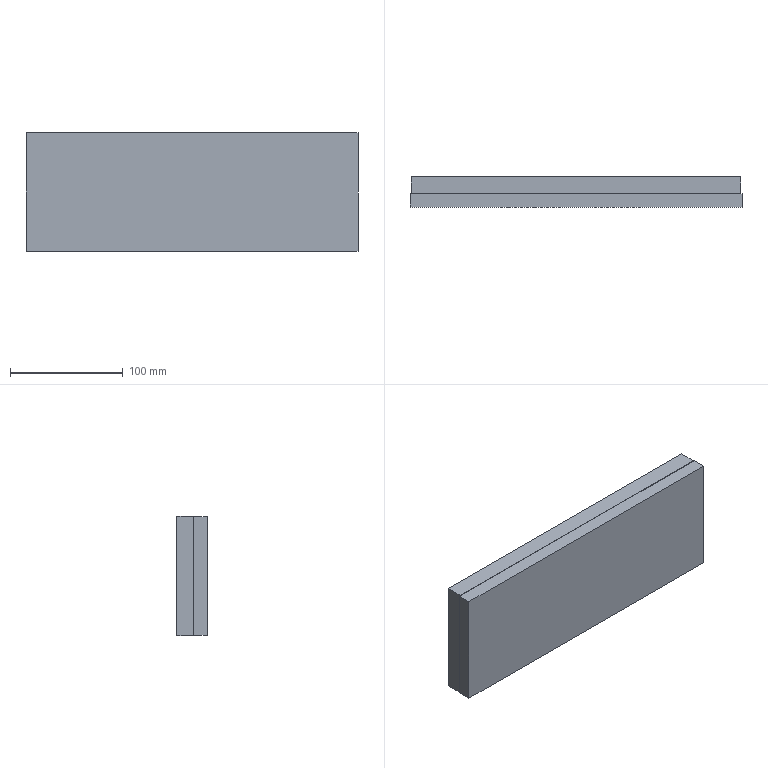NC program | NX | posted with a generic post | part box 295 x 27 x 106 mm
Lines 1811 to 3309 of 7486:
(FLOOR_WALL_3_COPY , TOOL : D8R0精铣)
N3566 T03 M6
N3568 G54
N3570 G17 G0 G90 X-101.999 Y-46.5 S3500 M3
N3572 G43 Z20. H3
N3574 Z3.
N3576 G94 G1 Z0. F600.
N3578 Y-42.99
N3580 X-102.002 Y36.988
N3582 G2 X-96.202 Y39.326 R14.
N3584 G1 X-96.199 Y-45.326
N3586 X-90.398 Y-50.129
N3588 X-90.402 Y44.124
N3590 G2 X-84.602 Y48.831 R14.
N3592 G1 X-84.598 Y-54.832
N3594 G3 X-79. Y-56. R14.
N3596 G1 X-78.797
N3598 X-78.801 Y50.
N3600 X-73.001
N3602 X-72.997 Y-56.
N3604 X-67.196
N3606 X-67.2 Y50.
N3608 X-67.201 Y53.
N3610 Z3.
N3612 G0 Z20.
N3614 X128. Y-59.
N3616 Z3.
N3618 G1 Z0.
N3620 Y-56.
N3622 Y50.
N3624 X133.534
N3626 Y-56.
N3628 X139.067
N3630 Y50.
N3632 X141.
N3634 G2 X144.6 Y49.529 R14.
N3636 G1 Y-55.529
N3638 G3 X150.133 Y-52.61 R14.
N3640 G1 Y46.61
N3642 X151.245 Y45.542
N3644 X152.232 Y44.357
N3646 X153.083 Y43.072
N3648 X153.787 Y41.7
N3650 X155.667 Y37.99
N3652 Y-43.99
N3654 X161.2 Y-41.499
N3656 Y35.499
N3658 G2 X166.733 Y31.489 R14.
N3660 G1 Y-37.489
N3662 G3 X169.906 Y-30.123 R14.
N3664 G1 X172.266 Y-11.5
N3666 Y5.5
N3668 X177.8
N3670 Y-11.5
N3672 Y-14.5
N3674 Z3.
N3676 G0 Z20.
(FLOOR_WALL_3 , TOOL : D8R0精铣)
N3678 X-59.697 Y-59.
N3680 Z2.75
N3682 G1 Z-0.25
N3684 Y-56.
N3686 Y50.
N3688 X-53.845
N3690 Y-56.
N3692 X-47.994
N3694 Y50.
N3696 X-42.142
N3698 Y-56.
N3700 X-36.291
N3702 Y50.
N3704 X-30.439
N3706 Y-56.
N3708 X-24.588
N3710 Y50.
N3712 X-18.736
N3714 Y-56.
N3716 X-12.885
N3718 Y50.
N3720 X-7.033
N3722 Y-56.
N3724 X-1.182
N3726 Y50.
N3728 X4.67
N3730 Y-56.
N3732 X10.521
N3734 Y50.
N3736 X16.373
N3738 Y-56.
N3740 X22.224
N3742 Y50.
N3744 X28.076
N3746 Y-56.
N3748 X33.927
N3750 Y50.
N3752 X39.779
N3754 Y-56.
N3756 X45.63
N3758 Y50.
N3760 X51.482
N3762 Y-56.
N3764 X57.333
N3766 Y50.
N3768 X63.185
N3770 Y-56.
N3772 X69.036
N3774 Y50.
N3776 X74.888
N3778 Y-56.
N3780 X80.739
N3782 Y50.
N3784 X86.591
N3786 Y-56.
N3788 X92.442
N3790 Y50.
N3792 X98.294
N3794 Y-56.
N3796 X104.145
N3798 Y50.
N3800 X109.997
N3802 Y-56.
N3804 X115.848
N3806 Y50.
N3808 X121.7
N3810 Y-56.
N3812 Y-59.
N3814 Z2.75
N3816 G0 Z20.
N3818 X-59.697
N3820 Z2.5
N3822 G1 Z-0.5
N3824 Y-56.
N3826 Y50.
N3828 X-53.845
N3830 Y-56.
N3832 X-47.994
N3834 Y50.
N3836 X-42.142
N3838 Y-56.
N3840 X-36.291
N3842 Y50.
N3844 X-30.439
N3846 Y-56.
N3848 X-24.588
N3850 Y50.
N3852 X-18.736
N3854 Y-56.
N3856 X-12.885
N3858 Y50.
N3860 X-7.033
N3862 Y-56.
N3864 X-1.182
N3866 Y50.
N3868 X4.67
N3870 Y-56.
N3872 X10.521
N3874 Y50.
N3876 X16.373
N3878 Y-56.
N3880 X22.224
N3882 Y50.
N3884 X28.076
N3886 Y-56.
N3888 X33.927
N3890 Y50.
N3892 X39.779
N3894 Y-56.
N3896 X45.63
N3898 Y50.
N3900 X51.482
N3902 Y-56.
N3904 X57.333
N3906 Y50.
N3908 X63.185
N3910 Y-56.
N3912 X69.036
N3914 Y50.
N3916 X74.888
N3918 Y-56.
N3920 X80.739
N3922 Y50.
N3924 X86.591
N3926 Y-56.
N3928 X92.442
N3930 Y50.
N3932 X98.294
N3934 Y-56.
N3936 X104.145
N3938 Y50.
N3940 X109.997
N3942 Y-56.
N3944 X115.848
N3946 Y50.
N3948 X121.7
N3950 Y-56.
N3952 Y-59.
N3954 Z2.5
N3956 G0 Z20.
(FLOOR_WALL_4 , TOOL : D8R0精铣)
N3958 X-53.5 Y3. S4500
N3960 Z2.55
N3962 G1 Z-0.45 F1000.
N3964 X-59.7
N3966 G3 X-39.471 Y-41.79 R59.7
N3968 G1 X-39.2 Y-42.029
N3970 Y-46.8
N3972 X-60.031
N3974 G3 X-59.95 Y-46. R4.
N3976 G1 Y-34.495
N3978 X-53.95
N3980 G3 X-48.97 Y-40.8 R65.7
N3982 G1 X-44.962 Y-42.521
N3984 X-48.97 Y-40.8
N3986 X-53.95
N3988 Y-34.495
N3990 X-59.95
N3992 Y-33.
N3994 G3 X-69. Y-23.95 R9.05
N3996 G1 X-87.
N3998 G2 X-87.95 Y-23. R0.95
N4000 G1 Y-14.5
N4002 G3 X-97. Y-5.45 R9.05
N4004 G1 X-104.
N4006 G3 X-104.8 Y-5.531 R4.
N4008 G1 Y11.531
N4010 G3 X-104. Y11.45 R4.
N4012 G1 X-97.
N4014 G3 X-87.95 Y20.5 R9.05
N4016 G1 Y29.
N4018 G2 X-87. Y29.95 R0.95
N4020 G1 X-69.
N4022 G3 X-59.95 Y39. R9.05
N4024 G1 Y52.
N4026 G3 X-60.031 Y52.8 R4.
N4028 G1 X-39.2
N4030 Y48.029
N4032 X-39.471 Y47.79
N4034 G3 X-49.023 Y37.071 R59.7
N4036 G1 X-53.95 Y40.495
N4038 Y46.8
N4040 X-48.97
N4042 X-44.962 Y48.521
N4044 X-48.97 Y46.8
N4046 G3 X-53.95 Y40.495 R65.7
N4048 G1 X-56.087 Y37.114
N4050 G2 X-59.975 Y29.573 R13.05
N4052 X-58.428 Y28.375 R4.
N4054 X-54.179 Y36.502 R63.7
N4056 X-56.087 Y37.114 R4.
N4058 G1 X-53.95 Y40.495
N4060 X-49.023 Y37.071
N4062 G3 X-59.7 Y3. R59.7
N4064 G1 X-65.7
N4066 G3 X-61.577 Y-19.908 R65.7
N4068 G1 X-59.975 Y-23.573
N4070 G2 X-56.087 Y-31.114 R13.05
N4072 X-54.179 Y-30.502 R4.
N4074 X-58.428 Y-22.375 R63.7
N4076 X-59.975 Y-23.573 R4.
N4078 G1 X-61.577 Y-19.908
N4080 G3 X-69. Y-17.95 R15.05
N4082 G1 X-81.95
N4084 Y-14.5
N4086 G3 X-97. Y0.55 R15.05
N4088 G1 X-98.8
N4090 Y5.45
N4092 X-97.
N4094 G3 X-81.95 Y20.5 R15.05
N4096 G1 Y23.95
N4098 X-69.
N4100 G3 X-61.577 Y25.908 R15.05
N4102 X-65.7 Y3. R65.7
N4104 G1 X-71.7
N4106 G3 X-70.124 Y-11.95 R71.7
N4108 G1 X-76.105
N4110 G3 X-85.302 Y3. R21.05
N4112 G1 X-89.359
N4114 X-85.302
N4116 G3 X-76.105 Y17.95 R21.05
N4118 G1 X-70.124
N4120 G3 X-71.7 Y3. R71.7
N4122 G1 X-75.3
N4124 G3 X-75.035 Y-3.313 R75.3
N4126 X-79.64 Y3. R24.65
N4128 X-75.035 Y9.313 R24.65
N4130 X-75.3 Y3. R75.3
N4132 X-75.293 Y2. R75.3
N4134 G1 X-72.294 Y2.04
N4136 Z2.55
N4138 G0 Z20.
N4140 X53.5 Y3.
N4142 Z2.55
N4144 G1 Z-0.45
N4146 X59.7
N4148 G3 X39.471 Y47.79 R59.7
N4150 G1 X39.2 Y48.029
N4152 Y52.8
N4154 X122.031
N4156 G3 X121.95 Y52. R4.
N4158 G1 Y39.
N4160 G3 X131. Y29.95 R9.05
N4162 G1 X149.
N4164 G2 X149.95 Y29. R0.95
N4166 G1 Y20.5
N4168 G3 X159. Y11.45 R9.05
N4170 G1 X166.
N4172 G3 X166.8 Y11.531 R4.
N4174 G1 Y8.3
N4176 X180.331
N4178 X181.8 Y6.831
N4180 Y-0.831
N4182 X180.331 Y-2.3
N4184 X166.8
N4186 Y-5.531
N4188 G3 X166. Y-5.45 R4.
N4190 G1 X159.
N4192 G3 X149.95 Y-14.5 R9.05
N4194 G1 Y-23.
N4196 G2 X149. Y-23.95 R0.95
N4198 G1 X131.
N4200 G3 X121.95 Y-33. R9.05
N4202 G1 Y-46.
N4204 G3 X122.031 Y-46.8 R4.
N4206 G1 X39.2
N4208 Y-42.029
N4210 X39.471 Y-41.79
N4212 G3 X59.7 Y3. R59.7
N4214 G1 X65.7
N4216 G3 X48.97 Y46.8 R65.7
N4218 G1 X44.962 Y48.521
N4220 X48.97 Y46.8
N4222 X115.95
N4224 Y39.
N4226 G3 X131. Y23.95 R15.05
N4228 G1 X143.95
N4230 Y20.5
N4232 G3 X159. Y5.45 R15.05
N4234 G1 X161.52
N4236 G3 X163.988 Y3. R6.
N4238 G1 X167.77 Y1.7
N4240 X177.8
N4242 Y4.3
N4244 X167.77
N4246 G2 X167.77 Y1.7 R4.
N4248 G1 X163.988 Y3.
N4250 G3 X161.52 Y0.55 R6.
N4252 G1 X159.
N4254 G3 X143.95 Y-14.5 R15.05
N4256 G1 Y-17.95
N4258 X131.
N4260 G3 X115.95 Y-33. R15.05
N4262 G1 Y-40.8
N4264 X48.97
N4266 X44.962 Y-42.521
N4268 X48.97 Y-40.8
N4270 G3 X65.7 Y3. R65.7
N4272 G1 X71.7
N4274 G3 X60.927 Y40.8 R71.7
N4276 G1 X57.345 Y42.735
N4278 X60.927 Y40.8
N4280 X109.95
N4282 Y39.
N4284 G3 X131. Y17.95 R21.05
N4286 G1 X138.105
N4288 G3 X147.302 Y3. R21.05
N4290 G1 X151.359
N4292 X147.302
N4294 G3 X138.105 Y-11.95 R21.05
N4296 G1 X131.
N4298 G3 X109.95 Y-33. R21.05
N4300 G1 Y-34.8
N4302 X60.927
N4304 X57.345 Y-36.735
N4306 X60.927 Y-34.8
N4308 G3 X71.7 Y3. R71.7
N4310 G1 X77.7
N4312 G3 X70.895 Y34.8 R77.7
N4314 G1 X104.278
N4316 G3 X131. Y11.95 R27.05
N4318 G1 X133.337
N4320 G3 X138.374 Y3. R27.05
N4322 X133.337 Y-5.95 R27.05
N4324 G1 X131.
N4326 G3 X104.278 Y-28.8 R27.05
N4328 G1 X70.895
N4330 G3 X77.7 Y3. R77.7
N4332 G1 X83.7
N4334 G3 X79.624 Y28.8 R83.7
N4336 G1 X99.563
N4338 G3 X129.304 Y5.994 R33.05
N4340 X130.963 Y3. R33.05
N4342 X129.304 Y0.006 R33.05
N4344 X99.563 Y-22.8 R33.05
N4346 G1 X79.624
N4348 G3 X83.7 Y3. R83.7
N4350 G1 X89.7
N4352 G3 X87.487 Y22.8 R89.7
N4354 G1 X95.469
N4356 G3 X115.87 Y3. R39.05
N4358 G1 X120.63
N4360 X115.87
N4362 G3 X95.469 Y-16.8 R39.05
N4364 G1 X87.487
N4366 G3 X89.7 Y3. R89.7
N4368 G1 X95.7
N4370 G3 X95.322 Y11.493 R95.7
N4372 G1 X93.4 Y16.645
N4374 X95.322 Y11.493
N4376 G3 X103.917 Y3. R45.05
N4378 X95.322 Y-5.493 R45.05
N4380 G1 X93.4 Y-10.645
N4382 X95.322 Y-5.493
N4384 G3 X95.7 Y3. R95.7
N4386 X95.695 Y4. R95.7
N4388 G1 X92.695 Y3.969
N4390 Z2.55
N4392 G0 Z20.
(FLOOR_WALL_4_COPY , TOOL : D8R0精铣)
N4394 X-53.5 Y3. S3500
N4396 Z2.5
N4398 G1 Z-0.5 F800.
N4400 X-59.7
N4402 G3 X-39.471 Y-41.79 R59.7
N4404 G1 X-39.2 Y-42.029
N4406 Y-46.8
N4408 X-60.081
N4410 G3 X-60. Y-46. R4.
N4412 G1 Y-34.423
N4414 X-54.
N4416 G3 X-48.97 Y-40.8 R65.7
N4418 G1 X-44.962 Y-42.521
N4420 X-48.97 Y-40.8
N4422 X-54.
N4424 Y-34.423
N4426 X-60.
N4428 Y-33.
N4430 G3 X-69. Y-24. R9.
N4432 G1 X-87.
N4434 G2 X-88. Y-23. R1.
N4436 G1 Y-14.5
N4438 G3 X-97. Y-5.5 R9.
N4440 G1 X-104.
N4442 G3 X-104.8 Y-5.581 R4.
N4444 G1 Y11.581
N4446 G3 X-104. Y11.5 R4.
N4448 G1 X-97.
N4450 G3 X-88. Y20.5 R9.
N4452 G1 Y29.
N4454 G2 X-87. Y30. R1.
N4456 G1 X-69.
N4458 G3 X-60. Y39. R9.
N4460 G1 Y52.
N4462 G3 X-60.081 Y52.8 R4.
N4464 G1 X-39.2
N4466 Y48.029
N4468 X-39.471 Y47.79
N4470 G3 X-49.068 Y37.005 R59.7
N4472 G1 X-54. Y40.423
N4474 Y46.8
N4476 X-48.97
N4478 X-44.962 Y48.521
N4480 X-48.97 Y46.8
N4482 G3 X-54. Y40.423 R65.7
N4484 G1 X-56.147 Y37.048
N4486 G2 X-59.964 Y29.654 R13.
N4488 X-58.398 Y28.444 R4.
N4490 X-54.223 Y36.429 R63.7
N4492 X-56.147 Y37.048 R4.
N4494 G1 X-54. Y40.423
N4496 X-49.068 Y37.005
N4498 G3 X-59.7 Y3. R59.7
N4500 G1 X-65.7
N4502 G3 X-61.55 Y-19.981 R65.7
N4504 G1 X-59.964 Y-23.654
N4506 G2 X-56.147 Y-31.048 R13.
N4508 X-54.223 Y-30.429 R4.
N4510 X-58.398 Y-22.444 R63.7
N4512 X-59.964 Y-23.654 R4.
N4514 G1 X-61.55 Y-19.981
N4516 G3 X-69. Y-18. R15.
N4518 G1 X-82.
N4520 Y-14.5
N4522 G3 X-97. Y0.5 R15.
N4524 G1 X-98.8
N4526 Y5.5
N4528 X-97.
N4530 G3 X-82. Y20.5 R15.
N4532 G1 Y24.
N4534 X-69.
N4536 G3 X-61.55 Y25.981 R15.
N4538 X-65.7 Y3. R65.7
N4540 G1 X-71.7
N4542 G3 X-70.113 Y-12. R71.7
N4544 G1 X-76.149
N4546 G3 X-85.392 Y3. R21.
N4548 G1 X-89.461
N4550 X-85.392
N4552 G3 X-76.149 Y18. R21.
N4554 G1 X-70.113
N4556 G3 X-71.7 Y3. R71.7
N4558 G1 X-75.3
N4560 G3 X-75.024 Y-3.446 R75.3
N4562 X-79.711 Y3. R24.6
N4564 X-75.024 Y9.446 R24.6
N4566 X-75.3 Y3. R75.3
N4568 X-75.293 Y2. R75.3
N4570 G1 X-72.294 Y2.04
N4572 Z2.5
N4574 G0 Z20.
N4576 X53.5 Y3.
N4578 Z2.5
N4580 G1 Z-0.5
N4582 X59.7
N4584 G3 X39.471 Y47.79 R59.7
N4586 G1 X39.2 Y48.029
N4588 Y52.8
N4590 X122.081
N4592 G3 X122. Y52. R4.
N4594 G1 Y39.
N4596 G3 X131. Y30. R9.
N4598 G1 X149.
N4600 G2 X150. Y29. R1.
N4602 G1 Y20.5
N4604 G3 X159. Y11.5 R9.
N4606 G1 X166.
N4608 G3 X166.8 Y11.581 R4.
N4610 G1 Y8.3
N4612 X180.331
N4614 X181.8 Y6.831
N4616 Y-0.831
N4618 X180.331 Y-2.3
N4620 X166.8
N4622 Y-5.581
N4624 G3 X166. Y-5.5 R4.
N4626 G1 X159.
N4628 G3 X150. Y-14.5 R9.
N4630 G1 Y-23.
N4632 G2 X149. Y-24. R1.
N4634 G1 X131.
N4636 G3 X122. Y-33. R9.
N4638 G1 Y-46.
N4640 G3 X122.081 Y-46.8 R4.
N4642 G1 X39.2
N4644 Y-42.029
N4646 X39.471 Y-41.79
N4648 G3 X59.7 Y3. R59.7
N4650 G1 X65.7
N4652 G3 X48.97 Y46.8 R65.7
N4654 G1 X44.962 Y48.521
N4656 X48.97 Y46.8
N4658 X116.
N4660 Y39.
N4662 G3 X131. Y24. R15.
N4664 G1 X144.
N4666 Y20.5
N4668 G3 X159. Y5.5 R15.
N4670 G1 X161.493
N4672 G3 X163.988 Y3. R6.
N4674 G1 X167.77 Y1.7
N4676 X177.8
N4678 Y4.3
N4680 X167.77
N4682 G2 X167.77 Y1.7 R4.
N4684 G1 X163.988 Y3.
N4686 G3 X161.493 Y0.5 R6.
N4688 G1 X159.
N4690 G3 X144. Y-14.5 R15.
N4692 G1 Y-18.
N4694 X131.
N4696 G3 X116. Y-33. R15.
N4698 G1 Y-40.8
N4700 X48.97
N4702 X44.962 Y-42.521
N4704 X48.97 Y-40.8
N4706 G3 X65.7 Y3. R65.7
N4708 G1 X71.7
N4710 G3 X60.927 Y40.8 R71.7
N4712 G1 X57.345 Y42.735
N4714 X60.927 Y40.8
N4716 X110.
N4718 Y39.
N4720 G3 X131. Y18. R21.
N4722 G1 X138.149
N4724 G3 X147.392 Y3. R21.
N4726 G1 X151.461
N4728 X147.392
N4730 G3 X138.149 Y-12. R21.
N4732 G1 X131.
N4734 G3 X110. Y-33. R21.
N4736 G1 Y-34.8
N4738 X60.927
N4740 X57.345 Y-36.735
N4742 X60.927 Y-34.8
N4744 G3 X71.7 Y3. R71.7
N4746 G1 X77.7
N4748 G3 X70.895 Y34.8 R77.7
N4750 G1 X104.329
N4752 G3 X131. Y12. R27.
N4754 G1 X133.373
N4756 G3 X138.439 Y3. R27.
N4758 X133.373 Y-6. R27.
N4760 G1 X131.
N4762 G3 X104.329 Y-28.8 R27.
N4764 G1 X70.895
N4766 G3 X77.7 Y3. R77.7
N4768 G1 X83.7
N4770 G3 X79.624 Y28.8 R83.7
N4772 G1 X99.616
N4774 G3 X129.336 Y6.042 R33.
N4776 X131.022 Y3. R33.
N4778 X129.336 Y-0.042 R33.
N4780 X99.616 Y-22.8 R33.
N4782 G1 X79.624
N4784 G3 X83.7 Y3. R83.7
N4786 G1 X89.7
N4788 G3 X87.487 Y22.8 R89.7
N4790 G1 X95.524
N4792 G3 X116. Y3. R39.
N4794 G1 X120.786
N4796 X116.
N4798 G3 X95.524 Y-16.8 R39.
N4800 G1 X87.487
N4802 G3 X89.7 Y3. R89.7
N4804 G1 X95.7
N4806 G3 X95.314 Y11.586 R95.7
N4808 G1 X93.401 Y16.718
N4810 X95.314 Y11.586
N4812 G3 X104. Y3. R45.
N4814 X95.314 Y-5.586 R45.
N4816 G1 X93.401 Y-10.718
N4818 X95.314 Y-5.586
N4820 G3 X95.7 Y3. R95.7
N4822 X95.695 Y4. R95.7
N4824 G1 X92.695 Y3.969
N4826 Z2.5
N4828 G0 Z20.
(FLOOR_WALL_5 , TOOL : D8R0精铣)
N4830 X-110.992 Y32.029
N4832 Z3.1
N4834 G1 Z0.1
N4836 X-110.791 Y31.75
N4838 G3 X-108. Y31.293 R2.
N4840 G1 X-73.607 Y56.
N4842 X-65.768
N4844 X-108. Y25.661
N4846 Y20.03
N4848 X-60. Y54.512
N4850 Y48.881
N4852 X-108. Y14.399
N4854 Y11.5
N4856 X-104.196
N4858 X-60. Y43.249
N4860 G3 X-59.543 Y46.041 R2.
N4862 G1 X-57.
N4864 Z3.1
N4866 G0 Z20.
N4868 X-71.419 Y-53.
N4870 Z3.1
N4872 G1 Z0.1
N4874 X-71.266 Y-52.761
N4876 G3 X-71.882 Y-50. R2.
N4878 G1 X-107.907 Y-27.112
N4880 G2 X-108. Y-25.5 R14.
N4882 G1 Y-21.635
N4884 X-63.353 Y-50.
N4886 X-60.
N4888 Y-46.712
N4890 X-108. Y-16.216
N4892 Y-10.798
N4894 X-60. Y-41.294
N4896 Y-35.875
N4898 X-107.81 Y-5.5
N4900 G3 X-110.57 Y-6.116 R2.
N4902 G1 X-111. Y-6.792
N4904 Z3.1
N4906 G0 Z20.
N4908 X119. Y-35.57
N4910 Z3.1
N4912 G1 Z0.1
N4914 X119.194 Y-35.821
N4916 G3 X122. Y-36.177 R2.
N4918 G1 X161.604 Y-5.5
N4920 X169.072
N4922 X122. Y-41.962
N4924 Y-47.748
N4926 X170. Y-10.567
N4928 Y-16.352
N4930 X126.561 Y-50.
N4932 X134.03
N4934 X170. Y-22.138
N4936 G3 X170.356 Y-19.332 R2.
N4938 G1 X173.
N4940 Z3.1
N4942 G0 Z20.
N4944 X168.036 Y8.5
N4946 Z3.1
N4948 G1 Z0.1
N4950 X168.188 Y8.739
N4952 G3 X167.572 Y11.5 R2.
N4954 G1 X122. Y40.453
N4956 Y45.872
N4958 X170. Y15.376
N4960 Y20.794
N4962 X122. Y51.29
N4964 Y56.
N4966 X123.116
N4968 X170. Y26.213
N4970 Y28.5
N4972 G3 X169.582 Y31.897 R14.
N4974 G1 X131.644 Y56.
N4976 G3 X128.884 Y55.384 R2.
N4978 G1 Y59.
N4980 Z3.1
N4982 G0 Z20.
(FLOOR_WALL_6 , TOOL : D8R0精铣)
N4984 X0. Y34.
N4986 Z-0.675
N4988 G1 Z-3.675
N4990 Y40.8
N4992 X-24.592
N4994 G2 X-27.633 Y36.645 R12.4
N4996 G1 X-29. Y35.423
N4998 G3 X-29. Y-29.423 R43.5
N5000 G1 X-27.633 Y-30.645
N5002 G2 X-24.592 Y-34.8 R12.4
N5004 G1 X-20.125
N5006 G3 X-17.582 Y-36.151 R40.2
N5008 G1 X-16.469 Y-36.743
N5010 X-17.582 Y-36.151
N5012 G2 X-20.125 Y-34.8 R40.2
N5014 X20.125 Y-34.8 R-40.2
N5016 X17.582 Y-36.151 R40.2
N5018 G1 X16.469 Y-36.743
N5020 X17.582 Y-36.151
N5022 G3 X20.125 Y-34.8 R40.2
N5024 G1 X24.592
N5026 G2 X27.633 Y-30.645 R12.4
N5028 G1 X29. Y-29.423
N5030 G3 X29. Y35.423 R43.5
N5032 G1 X27.634 Y36.645
N5034 G2 X24.592 Y40.8 R12.4
N5036 G1 X0.
N5038 Y46.8
N5040 X-29.5
N5042 Y45.888
N5044 G2 X-31.633 Y41.118 R6.4
N5046 G1 X-33. Y39.895
N5048 G3 X-33. Y-33.895 R49.5
N5050 G1 X-31.633 Y-35.118
N5052 G2 X-29.5 Y-39.888 R6.4
N5054 G1 Y-40.8
N5056 X29.5
N5058 Y-39.888
N5060 G2 X31.633 Y-35.118 R6.4
N5062 G1 X33. Y-33.895
N5064 G3 X33. Y39.895 R49.5
N5066 G1 X31.634 Y41.117
N5068 G2 X29.5 Y45.888 R6.4
N5070 G1 Y46.8
N5072 X0.
N5074 Y52.8
N5076 X-35.5
N5078 Y45.888
N5080 G2 X-35.633 Y45.59 R0.4
N5082 G1 X-37. Y44.367
N5084 G3 X-37. Y-38.367 R55.5
N5086 G1 X-35.633 Y-39.59
N5088 G2 X-35.5 Y-39.888 R0.4
N5090 G1 Y-46.8
N5092 X35.5
N5094 Y-39.888
N5096 G2 X35.633 Y-39.59 R0.4
N5098 G1 X37. Y-38.367
N5100 G3 X37. Y44.367 R55.5
N5102 G1 X35.634 Y45.589
N5104 G2 X35.5 Y45.888 R0.4
N5106 G1 Y52.8
N5108 X0.
N5110 X-1.
N5112 Y59.
N5114 Z-0.675
N5116 G0 Z20.
N5118 X-35.9 Y59.1
N5120 Z-0.675
N5122 G1 Z-3.675
N5124 Y52.8
N5126 Y45.888
N5128 X-37.267 Y44.665
N5130 G3 X-37.267 Y-38.665 R55.9
N5132 G1 X-35.9 Y-39.888
N5134 Y-46.8
N5136 Y-53.1
N5138 Z-0.675
N5140 G0 Z20.
N5142 X35.9
N5144 Z-0.675
N5146 G1 Z-3.675
N5148 Y-46.8
N5150 Y-39.888
N5152 X37.267 Y-38.665
N5154 G3 X37.267 Y44.665 R55.9
N5156 G1 X35.9 Y45.888
N5158 Y52.8
N5160 Y59.1
N5162 Z-0.675
N5164 G0 Z20.
N5166 X0. Y34.
N5168 Z-0.85
N5170 G1 Z-3.85
N5172 Y40.8
N5174 X-24.592
N5176 G2 X-27.633 Y36.645 R12.4
N5178 G1 X-29. Y35.423
N5180 G3 X-29. Y-29.423 R43.5
N5182 G1 X-27.633 Y-30.645
N5184 G2 X-24.592 Y-34.8 R12.4
N5186 G1 X-20.125
N5188 G3 X-17.582 Y-36.151 R40.2
N5190 G1 X-16.469 Y-36.743
N5192 X-17.582 Y-36.151
N5194 G2 X-20.125 Y-34.8 R40.2
N5196 X20.125 Y-34.8 R-40.2
N5198 X17.582 Y-36.151 R40.2
N5200 G1 X16.469 Y-36.743
N5202 X17.582 Y-36.151
N5204 G3 X20.125 Y-34.8 R40.2
N5206 G1 X24.592
N5208 G2 X27.633 Y-30.645 R12.4
N5210 G1 X29. Y-29.423
N5212 G3 X29. Y35.423 R43.5
N5214 G1 X27.634 Y36.645
N5216 G2 X24.592 Y40.8 R12.4
N5218 G1 X0.
N5220 Y46.8
N5222 X-29.5
N5224 Y45.888
N5226 G2 X-31.633 Y41.118 R6.4
N5228 G1 X-33. Y39.895
N5230 G3 X-33. Y-33.895 R49.5
N5232 G1 X-31.633 Y-35.118
N5234 G2 X-29.5 Y-39.888 R6.4
N5236 G1 Y-40.8
N5238 X29.5
N5240 Y-39.888
N5242 G2 X31.633 Y-35.118 R6.4
N5244 G1 X33. Y-33.895
N5246 G3 X33. Y39.895 R49.5
N5248 G1 X31.634 Y41.117
N5250 G2 X29.5 Y45.888 R6.4
N5252 G1 Y46.8
N5254 X0.
N5256 Y52.8
N5258 X-35.5
N5260 Y45.888
N5262 G2 X-35.633 Y45.59 R0.4
N5264 G1 X-37. Y44.367
N5266 G3 X-37. Y-38.367 R55.5
N5268 G1 X-35.633 Y-39.59
N5270 G2 X-35.5 Y-39.888 R0.4
N5272 G1 Y-46.8
N5274 X35.5
N5276 Y-39.888
N5278 G2 X35.633 Y-39.59 R0.4
N5280 G1 X37. Y-38.367
N5282 G3 X37. Y44.367 R55.5
N5284 G1 X35.634 Y45.589
N5286 G2 X35.5 Y45.888 R0.4
N5288 G1 Y52.8
N5290 X0.
N5292 X-1.
N5294 Y59.
N5296 Z-0.85
N5298 G0 Z20.
N5300 X-35.9 Y59.1
N5302 Z-0.85
N5304 G1 Z-3.85
N5306 Y52.8
N5308 Y45.888
N5310 X-37.267 Y44.665
N5312 G3 X-37.267 Y-38.665 R55.9
N5314 G1 X-35.9 Y-39.888
N5316 Y-46.8
N5318 Y-53.1
N5320 Z-0.85
N5322 G0 Z20.
N5324 X35.9
N5326 Z-0.85
N5328 G1 Z-3.85
N5330 Y-46.8
N5332 Y-39.888
N5334 X37.267 Y-38.665
N5336 G3 X37.267 Y44.665 R55.9
N5338 G1 X35.9 Y45.888
N5340 Y52.8
N5342 Y59.1
N5344 Z-0.85
N5346 G0 Z20.
(PLANAR_MILL_4 , TOOL : D8R0精铣)
N5348 X2. Y34.893
N5350 Z-7.
N5352 G1 Z-10.
N5354 Y34.95
N5356 G3 X0. Y36.95 R2.
N5358 X-36.95 Y0. R36.95
N5360 X0. Y36.95 R-36.95
N5362 X-2. Y34.95 R2.
N5364 G1 X2. Y35.
N5366 G3 X0. Y37. R2.
N5368 X-37. Y0. R37.
N5370 X0. Y37. R-37.
N5372 X-2. Y34.943 R2.001
N5374 G1 Z-7.
N5376 G0 Z20.
N5378 M5
(PLANAR_MILL_2_COPY , TOOL : DJ-D3倒角)
N5380 T07 M6
N5382 G54
N5384 G17 G0 G90 X133.5 Y53.9 S3500 M3
N5386 G43 Z20. H7
N5388 Z2.6
N5390 G94 G1 Z-0.4 F1000.
N5392 Y52.4
N5394 X141.
N5396 G2 X150.907 Y45.164 R10.4
N5398 G3 X158.107 Y38.684 R9.6
N5400 G2 X166.4 Y28.5 R10.4
N5402 G1 Y15.5
N5404 G2 X166. Y15.1 R0.4
N5406 G1 X159.
N5408 G2 X153.6 Y20.5 R5.4
N5410 G1 Y29.
N5412 G3 X149. Y33.6 R4.6
N5414 G1 X131.
N5416 G2 X125.6 Y39. R5.4
N5418 G1 Y52.
N5420 G2 X126. Y52.4 R0.4
N5422 G1 X133.5
N5424 Y53.9
N5426 Z2.6
N5428 G0 Z20.
N5430 Y-47.9
N5432 Z2.6
N5434 G1 Z-0.4
N5436 Y-46.4
N5438 X126.
N5440 G2 X125.6 Y-46. R0.4
N5442 G1 Y-33.
N5444 G2 X131. Y-27.6 R5.4
N5446 G1 X149.
N5448 G3 X153.6 Y-23. R4.6
N5450 G1 Y-14.5
N5452 G2 X159. Y-9.1 R5.4
N5454 G1 X166.
N5456 G2 X166.4 Y-9.5 R0.4
N5458 G1 Y-22.5
N5460 G2 X158.107 Y-32.684 R10.4
N5462 G3 X150.907 Y-39.164 R9.6
N5464 G2 X141. Y-46.4 R10.4
N5466 G1 X133.5
N5468 Y-47.9
N5470 Z2.6
N5472 G0 Z20.
N5474 X-71.5 Y53.9
N5476 Z2.6
N5478 G1 Z-0.4
N5480 Y52.4
N5482 X-64.
N5484 G2 X-63.6 Y52. R0.4
N5486 G1 Y39.
N5488 G2 X-69. Y33.6 R5.4
N5490 G1 X-87.
N5492 G3 X-91.6 Y29. R4.6
N5494 G1 Y20.5
N5496 G2 X-97. Y15.1 R5.4
N5498 G1 X-104.
N5500 G2 X-104.4 Y15.5 R0.4
N5502 G1 Y31.5
N5504 G2 X-95.403 Y41.805 R10.4
N5506 G3 X-88.203 Y46.845 R9.6
N5508 G2 X-79. Y52.4 R10.4
N5510 G1 X-71.5
N5512 Y53.9
N5514 Z2.6
N5516 G0 Z20.
N5518 X-105.9 Y-17.5
N5520 Z2.6
N5522 G1 Z-0.4
N5524 X-104.4
N5526 Y-9.5
N5528 G2 X-104. Y-9.1 R0.4
N5530 G1 X-97.
N5532 G2 X-91.6 Y-14.5 R5.4
N5534 G1 Y-23.
N5536 G3 X-87. Y-27.6 R4.6
N5538 G1 X-69.
N5540 G2 X-63.6 Y-33. R5.4
N5542 G1 Y-46.
N5544 G2 X-64. Y-46.4 R0.4
N5546 G1 X-79.
N5548 G2 X-88.203 Y-40.845 R10.4
N5550 G3 X-95.403 Y-35.805 R9.6
N5552 G2 X-104.4 Y-25.5 R10.4
N5554 G1 Y-17.5
N5556 X-105.9
N5558 Z2.6
N5560 G0 Z20.
(PLANAR_MILL_2_COPY_COPY , TOOL : DJ-D3倒角)
N5562 X161.905 Y21.219
N5564 Z1.5
N5566 G1 Z-0.5
N5568 G3 X162.78 Y22.33 R1.
N5570 G1 X162.615 Y23.72
N5572 G3 X159.505 Y26.171 R2.8
N5574 X157.054 Y23.06 R2.8
N5576 G1 X157.385 Y20.28
N5578 G3 X160.495 Y17.829 R2.8
N5580 X162.946 Y20.94 R2.8
N5582 G1 X162.78 Y22.33
N5584 G3 X161.67 Y23.205 R1.
N5586 G1 Z1.5
N5588 G0 Z20.
N5590 Y-17.205
N5592 Z1.5
N5594 G1 Z-0.5
N5596 G3 X162.78 Y-16.33 R1.
N5598 G1 X162.946 Y-14.94
N5600 G3 X160.495 Y-11.829 R2.8
N5602 X157.385 Y-14.28 R2.8
N5604 G1 X157.054 Y-17.06
N5606 G3 X159.505 Y-20.171 R2.8
N5608 X162.615 Y-17.72 R2.8
N5610 G1 X162.78 Y-16.33
N5612 G3 X161.905 Y-15.219 R1.
N5614 G1 Z1.5
N5616 G0 Z20.
N5618 X-99.953 Y-15.36
N5620 Z1.5
N5622 G1 Z-0.5
N5624 X-99.957 Y-15.361
N5626 G3 X-100.749 Y-16.533 R1.
N5628 G1 X-100.582 Y-17.392
N5630 G3 X-97.301 Y-19.608 R2.8
N5632 X-95.085 Y-16.326 R2.8
N5634 G1 X-95.418 Y-14.608
N5636 G3 X-98.699 Y-12.392 R2.8
N5638 X-100.915 Y-15.674 R2.8
N5640 G1 X-100.749 Y-16.533
N5642 G3 X-99.572 Y-17.323 R1.
N5644 G1 Z1.5
N5646 G0 Z20.
N5648 Y23.323
N5650 Z1.5
N5652 G1 Z-0.5
N5654 X-99.577 Y23.324
N5656 G3 X-100.749 Y22.533 R1.
N5658 G1 X-100.915 Y21.674
N5660 G3 X-98.699 Y18.392 R2.8
N5662 X-95.418 Y20.608 R2.8
N5664 G1 X-95.085 Y22.326
N5666 G3 X-97.301 Y25.608 R2.8
N5668 X-100.582 Y23.392 R2.8
N5670 G1 X-100.749 Y22.533
N5672 G3 X-99.953 Y21.36 R1.
N5674 G1 Z1.5
N5676 G0 Z20.
(PLANAR_MILL_3_COPY , TOOL : DJ-D3倒角)
N5678 X-107. Y-9.5
N5680 Z1.5
N5682 G1 Z-1.5
N5684 G3 X-105. Y-7.5 R2.
N5686 G1 Y13.5
N5688 G3 X-107. Y15.5 R2.
N5690 G1 Z1.5
N5692 G0 Z20.
N5694 X-64. Y55.
N5696 Z1.5
N5698 G1 Z-1.5
N5700 G3 X-62. Y53. R2.
N5702 G1 X-40.
N5704 G2 X-39. Y52. R1.
N5706 G1 Y47.721
N5708 G2 X-39.333 Y46.976 R1.
N5710 G3 X-39.333 Y-40.976 R59.
N5712 G2 X-39. Y-41.721 R1.
N5714 G1 Y-46.
N5716 G2 X-40. Y-47. R1.
N5718 G1 X-62.
N5720 G3 X-64. Y-49. R2.
N5722 G1 Z1.5
N5724 G0 Z20.
N5726 X126.
N5728 Z1.5
N5730 G1 Z-1.5
N5732 G3 X124. Y-47. R2.
N5734 G1 X40.
N5736 G2 X39. Y-46. R1.
N5738 G1 Y-41.721
N5740 G2 X39.333 Y-40.976 R1.
N5742 G3 X39.333 Y46.976 R59.
N5744 G2 X39. Y47.721 R1.
N5746 G1 Y52.
N5748 G2 X40. Y53. R1.
N5750 G1 X124.
N5752 G3 X126. Y55. R2.
N5754 G1 Z1.5
N5756 G0 Z20.
N5758 X169. Y15.5
N5760 Z1.5
N5762 G1 Z-1.5
N5764 G3 X167. Y13.5 R2.
N5766 G1 Y9.5
N5768 G3 X168. Y8.5 R1.
N5770 G1 X180.
N5772 G2 X180.707 Y8.207 R1.
N5774 G1 X181.707 Y7.207
N5776 G2 X182. Y6.5 R1.
N5778 G1 Y-0.5
N5780 G2 X181.707 Y-1.207 R1.
N5782 G1 X180.707 Y-2.207
N5784 G2 X180. Y-2.5 R1.
N5786 G1 X168.
N5788 G3 X167. Y-3.5 R1.
N5790 G1 Y-7.5
N5792 G3 X169. Y-9.5 R2.
N5794 G1 Z1.5
N5796 G0 Z20.
(PLANAR_MILL_5_COPY , TOOL : DJ-D3倒角)
N5798 X39.936 Y-48.5
N5800 Z-2.
N5802 G1 Z-5.
N5804 G3 X38. Y-47. R2.
N5806 G1 X-38.
N5808 G3 X-39.936 Y-48.5 R2.
N5810 G1 Z-2.
N5812 G0 Z20.
N5814 Y54.5
N5816 Z-2.
N5818 G1 Z-5.
N5820 G3 X-38. Y53. R2.
N5822 G1 X38.
N5824 G3 X39.936 Y54.5 R2.
N5826 G1 Z-2.
N5828 G0 Z20.
(PLANAR_MILL_5 , TOOL : DJ-D3倒角)
N5830 X1.949 Y38.451
N5832 Z-2.
N5834 G1 Z-5.
N5836 G3 X0. Y40. R2.
N5838 X-40. Y0. R40.
N5840 X0. Y40. R-40.
N5842 X-1.949 Y38.451 R2.
N5844 G1 Z-2.
N5846 G0 Z20.
N5848 M5
(FLOOR_WALL_3_COPY_1_COPY , TOOL : D8R0精铣)
N5850 T03 M6
N5852 G54
N5854 G17 G0 G90 X44.003 Y-7. S3500 M3
N5856 G43 Z20. H3
N5858 Z2.5
N5860 G94 G1 Z-0.5 F800.
N5862 Y-4.
N5864 Y101.6
N5866 G2 X44.403 Y102. R0.4
N5868 G1 X49.474
N5870 G2 X49.874 Y101.6 R0.4
N5872 G1 Y-3.6
N5874 G3 X50.273 Y-4. R0.4
N5876 G1 X55.345
N5878 G3 X55.745 Y-3.6 R0.4
N5880 G1 Y101.6
N5882 G2 X56.144 Y102. R0.4
N5884 G1 X61.216
N5886 G2 X61.616 Y101.6 R0.4
N5888 G1 Y-3.6
N5890 G3 X62.015 Y-4. R0.4
N5892 G1 X67.087
N5894 G3 X67.486 Y-3.6 R0.4
N5896 G1 Y101.6
N5898 G2 X67.886 Y102. R0.4
N5900 G1 X72.958
N5902 G2 X73.357 Y101.6 R0.4
N5904 G1 Y-3.6
N5906 G3 X73.757 Y-4. R0.4
N5908 G1 X78.829
N5910 G3 X79.228 Y-3.6 R0.4
N5912 G1 Y101.6
N5914 G2 X79.628 Y102. R0.4
N5916 G1 X84.7
N5918 G2 X85.099 Y101.6 R0.4
N5920 G1 Y-3.6
N5922 G3 X85.499 Y-4. R0.4
N5924 G1 X90.57
N5926 G3 X90.97 Y-3.6 R0.4
N5928 G1 Y101.6
N5930 G2 X91.37 Y102. R0.4
N5932 G1 X96.441
N5934 G2 X96.841 Y101.6 R0.4
N5936 G1 Y-3.6
N5938 G3 X97.24 Y-4. R0.4
N5940 G1 X102.312
N5942 G3 X102.712 Y-3.6 R0.4
N5944 G1 Y101.6
N5946 G2 X103.111 Y102. R0.4
N5948 G1 X108.183
N5950 G2 X108.583 Y101.6 R0.4
N5952 G1 Y-3.6
N5954 G3 X108.982 Y-4. R0.4
N5956 G1 X114.054
N5958 G3 X114.453 Y-3.6 R0.4
N5960 G1 Y101.6
N5962 G2 X114.853 Y102. R0.4
N5964 G1 X119.925
N5966 G2 X120.324 Y101.6 R0.4
N5968 G1 Y-3.6
N5970 G3 X120.724 Y-4. R0.4
N5972 G1 X125.796
N5974 G3 X126.195 Y-3.6 R0.4
N5976 G1 Y101.6
N5978 G2 X126.595 Y102. R0.4
N5980 G1 X131.667
N5982 G2 X132.066 Y101.6 R0.4
N5984 G1 Y-3.6
N5986 G3 X132.466 Y-4. R0.4
N5988 G1 X137.537
N5990 G3 X137.937 Y-3.6 R0.4
N5992 G1 Y101.6
N5994 G2 X138.336 Y102. R0.4
N5996 G1 X143.408
N5998 G2 X143.808 Y101.6 R0.4
N6000 G1 Y-3.6
N6002 G3 X144.207 Y-4. R0.4
N6004 G1 X149.279
N6006 G3 X149.679 Y-3.6 R0.4
N6008 G1 Y101.6
N6010 G2 X150.078 Y102. R0.4
N6012 G1 X155.15
N6014 G2 X155.55 Y101.6 R0.4
N6016 G1 Y-3.6
N6018 G3 X155.949 Y-4. R0.4
N6020 G1 X161.021
N6022 G3 X161.42 Y-3.6 R0.4
N6024 G1 Y101.6
N6026 G2 X161.82 Y102. R0.4
N6028 G1 X166.892
N6030 G2 X167.291 Y101.6 R0.4
N6032 G1 Y-3.6
N6034 G3 X167.691 Y-4. R0.4
N6036 G1 X172.763
N6038 G3 X173.162 Y-3.6 R0.4
N6040 G1 Y101.6
N6042 G2 X173.562 Y102. R0.4
N6044 G1 X178.634
N6046 G2 X179.033 Y101.6 R0.4
N6048 G1 Y-3.6
N6050 G3 X179.433 Y-4. R0.4
N6052 G1 X184.504
N6054 G3 X184.904 Y-3.6 R0.4
N6056 G1 Y101.6
N6058 G2 X185.303 Y102. R0.4
N6060 G1 X190.375
N6062 G2 X190.775 Y101.6 R0.4
N6064 G1 Y-3.6
N6066 G3 X191.174 Y-4. R0.4
N6068 G1 X196.246
N6070 G3 X196.646 Y-3.6 R0.4
N6072 G1 Y101.6
N6074 G2 X197.045 Y102. R0.4
N6076 G1 X202.117
N6078 G2 X202.517 Y101.6 R0.4
N6080 G1 Y-3.6
N6082 G3 X202.916 Y-4. R0.4
N6084 G1 X207.988
N6086 G3 X208.387 Y-3.6 R0.4
N6088 G1 Y101.6
N6090 G2 X208.787 Y102. R0.4
N6092 G1 X213.859
N6094 G2 X214.258 Y101.6 R0.4
N6096 G1 Y-3.6
N6098 G3 X214.658 Y-4. R0.4
N6100 G1 X219.73
N6102 G3 X220.129 Y-3.6 R0.4
N6104 G1 Y101.6
N6106 G2 X220.529 Y102. R0.4
N6108 G1 X225.6
N6110 G2 X226. Y101.6 R0.4
N6112 G1 Y-4.
N6114 Y-7.
N6116 Z2.5
N6118 G0 Z20.
(FLOOR_WALL_3_COPY_COPY , TOOL : D8R0精铣)
N6120 X2.001 Y5.5
N6122 Z3.03
N6124 G1 Z0.03 F1000.
N6126 Y9.01
N6128 X1.998 Y88.777
N6130 G2 X2.174 Y89.108 R0.4
N6132 X7.419 Y91.26 R14.
N6134 X7.798 Y90.946 R0.32
N6136 G1 X7.801 Y6.861
N6138 G3 X7.946 Y6.554 R0.4
N6140 G1 X13.34 Y2.088
N6142 G3 X13.602 Y2.211 R0.16
N6144 G1 X13.598 Y95.996
N6146 G2 X13.674 Y96.23 R0.4
N6148 X19.057 Y100.676 R14.
N6150 X19.398 Y100.459 R0.24
N6152 G1 X19.402 Y-2.568
N6154 G3 X19.649 Y-2.937 R0.4
N6156 X24.839 Y-3.999 R14.
N6158 X25.203 Y-3.64 R0.36
N6160 G1 X25.199 Y101.6
N6162 G2 X25.598 Y102. R0.4
N6164 G1 X30.6
N6166 G2 X30.999 Y101.601 R0.4
N6168 G1 X31.003 Y-3.6
N6170 G3 X31.403 Y-4. R0.4
N6172 G1 X36.404
N6174 G3 X36.804 Y-3.6 R0.4
N6176 G1 X36.8 Y102.
N6178 X36.799 Y105.
N6180 Z3.03
N6182 G0 Z20.
N6184 X232. Y-7.
N6186 Z3.03
N6188 G1 Z0.03
N6190 Y-4.
N6192 Y101.6
N6194 G2 X232.4 Y102. R0.4
N6196 G1 X237.134
N6198 G2 X237.534 Y101.6 R0.4
N6200 G1 Y-3.6
N6202 G3 X237.933 Y-4. R0.4
N6204 G1 X242.667
N6206 G3 X243.067 Y-3.6 R0.4
N6208 G1 Y101.6
N6210 G2 X243.466 Y102. R0.4
N6212 G1 X245.
N6214 G2 X248.295 Y101.607 R14.
N6216 X248.6 Y101.219 R0.4
N6218 G1 Y-3.16
N6220 G3 X248.959 Y-3.429 R0.28
N6222 X253.991 Y-0.732 R14.
N6224 X254.133 Y-0.426 R0.4
N6226 G1 Y98.235
N6228 G2 X254.404 Y98.35 R0.16
N6230 G1 X255.229 Y97.557
N6232 X255.259 Y97.525
N6234 X256.218 Y96.374
N6236 X256.244 Y96.339
N6238 X257.071 Y95.09
N6240 X257.093 Y95.052
N6242 X257.787 Y93.701
N6244 Y93.699
N6246 X259.624 Y90.075
N6248 X259.685 Y89.994
N6250 X259.667 Y89.895
N6252 Y8.381
N6254 G3 X260.005 Y8.162 R0.24
N6256 G1 X264.965 Y10.396
N6258 G3 X265.2 Y10.76 R0.4
N6260 G1 Y87.139
N6262 G2 X265.534 Y87.36 R0.24
N6264 X270.637 Y83.602 R14.
N6266 X270.733 Y83.343 R0.4
N6268 G1 Y14.847
N6270 G3 X270.947 Y14.773 R0.12
N6272 X273.905 Y21.875 R14.
N6274 G1 X273.906 Y21.879
N6276 X276.263 Y40.475
N6278 X276.266 Y40.525
N6280 Y57.1
N6282 G2 X276.666 Y57.5 R0.4
N6284 G1 X281.4
N6286 G2 X281.8 Y57.1 R0.4
N6288 G1 Y40.5
N6290 Y37.5
N6292 Z3.03
N6294 G0 Z20.
(FLOOR_WALL_3_COPY_COPY_COPY , TOOL : D8R0精铣)
N6296 X2.001 Y5.5 S4500
N6298 Z3.
N6300 G1 Z0. F800.
N6302 Y9.01
N6304 X1.998 Y88.777
N6306 G2 X2.174 Y89.108 R0.4
N6308 X7.419 Y91.26 R14.
N6310 X7.798 Y90.946 R0.32
N6312 G1 X7.801 Y6.861
N6314 G3 X7.946 Y6.554 R0.4
N6316 G1 X13.34 Y2.088
N6318 G3 X13.602 Y2.211 R0.16
N6320 G1 X13.598 Y95.996
N6322 G2 X13.674 Y96.23 R0.4
N6324 X19.057 Y100.676 R14.
N6326 X19.398 Y100.459 R0.24
N6328 G1 X19.402 Y-2.568
N6330 G3 X19.649 Y-2.937 R0.4
N6332 X24.839 Y-3.999 R14.
N6334 X25.203 Y-3.64 R0.36
N6336 G1 X25.199 Y101.6
N6338 G2 X25.598 Y102. R0.4
N6340 G1 X30.6
N6342 G2 X30.999 Y101.601 R0.4
N6344 G1 X31.003 Y-3.6
N6346 G3 X31.403 Y-4. R0.4
N6348 G1 X36.404
N6350 G3 X36.804 Y-3.6 R0.4
N6352 G1 X36.8 Y102.
N6354 X36.799 Y105.
N6356 Z3.
N6358 G0 Z20.
N6360 X232. Y-7.
N6362 Z3.
N6364 G1 Z0.
N6366 Y-4.
N6368 Y101.6
N6370 G2 X232.4 Y102. R0.4
N6372 G1 X237.134
N6374 G2 X237.534 Y101.6 R0.4
N6376 G1 Y-3.6
N6378 G3 X237.933 Y-4. R0.4
N6380 G1 X242.667
N6382 G3 X243.067 Y-3.6 R0.4
N6384 G1 Y101.6
N6386 G2 X243.466 Y102. R0.4
N6388 G1 X245.
N6390 G2 X248.295 Y101.607 R14.
N6392 X248.6 Y101.219 R0.4
N6394 G1 Y-3.16
N6396 G3 X248.959 Y-3.429 R0.28
N6398 X253.991 Y-0.732 R14.
N6400 X254.133 Y-0.426 R0.4
N6402 G1 Y98.235
N6404 G2 X254.404 Y98.35 R0.16
N6406 G1 X255.229 Y97.557
N6408 X255.259 Y97.525
N6410 X256.218 Y96.374
N6412 X256.244 Y96.339
N6414 X257.071 Y95.09
N6416 X257.093 Y95.052
N6418 X257.787 Y93.701
N6420 Y93.699
N6422 X259.624 Y90.075
N6424 X259.685 Y89.994
N6426 X259.667 Y89.895
N6428 Y8.381
N6430 G3 X260.005 Y8.162 R0.24
N6432 G1 X264.965 Y10.396
N6434 G3 X265.2 Y10.76 R0.4
N6436 G1 Y87.139
N6438 G2 X265.534 Y87.36 R0.24
N6440 X270.637 Y83.602 R14.
N6442 X270.733 Y83.343 R0.4
N6444 G1 Y14.847
N6446 G3 X270.947 Y14.773 R0.12
N6448 X273.905 Y21.875 R14.
N6450 G1 X273.906 Y21.879
N6452 X276.263 Y40.475
N6454 X276.266 Y40.525
N6456 Y57.1
N6458 G2 X276.666 Y57.5 R0.4
N6460 G1 X281.4
N6462 G2 X281.8 Y57.1 R0.4
N6464 G1 Y40.5
N6466 Y37.5
N6468 Z3.
N6470 G0 Z20.
N6472 M5